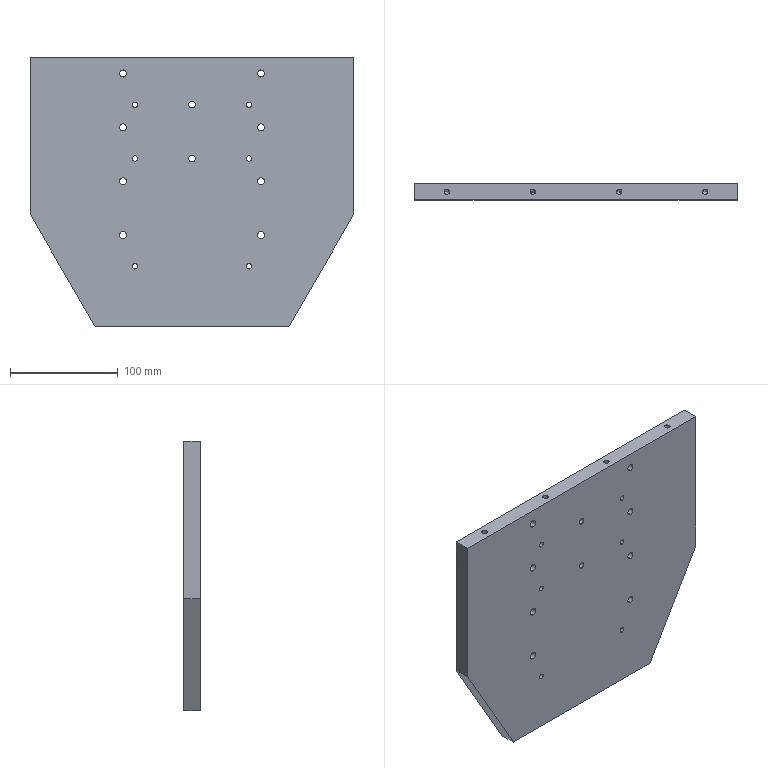Part | STEP file | KF-2212-060-002 | 1 solid | 80 faces | box 300 x 15 x 250 mm | volume 1020222 mm3 | cylinder 56 | plane 16 | cone 8 | commonest cylinder face diameters 5 x20 6.6 x16 11 x16 6 x4